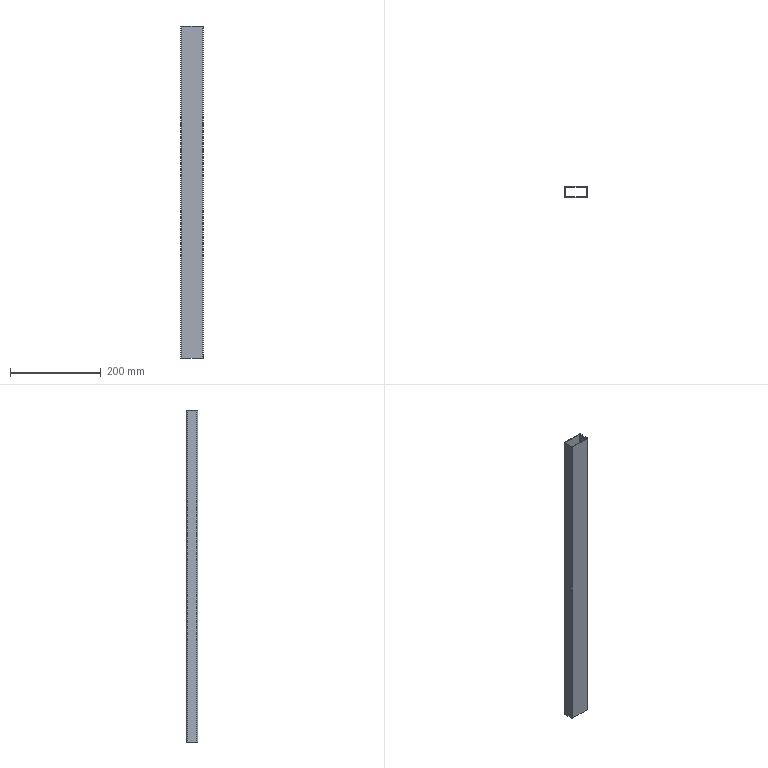Part | STEP file | PN_0025_default | 1 solid | 20 faces | box 50 x 25 x 730 mm | volume 154272 mm3 | plane 10 | cylinder 10 | commonest cylinder face diameters 2 x4 5 x4 10 x2